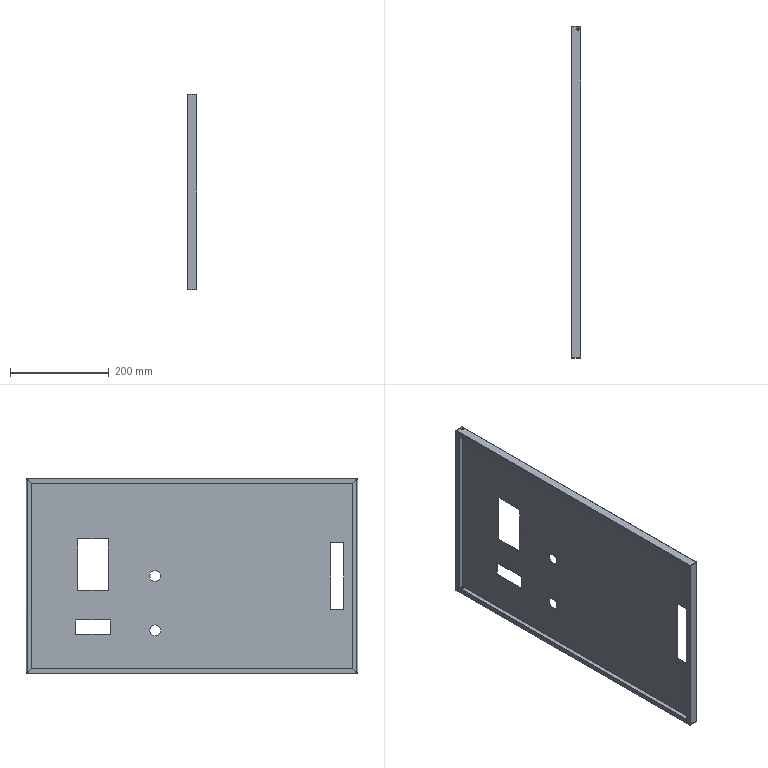Part | SolidWorks | features BaseBody 1 | 1 solid | 106 faces | box 20 x 671 x 396 mm | volume 462181 mm3 | plane 74 | cylinder 24 | spline 8 | commonest cylinder face diameters 0.4 x8 3.4 x8 5.1 x4 22 x4